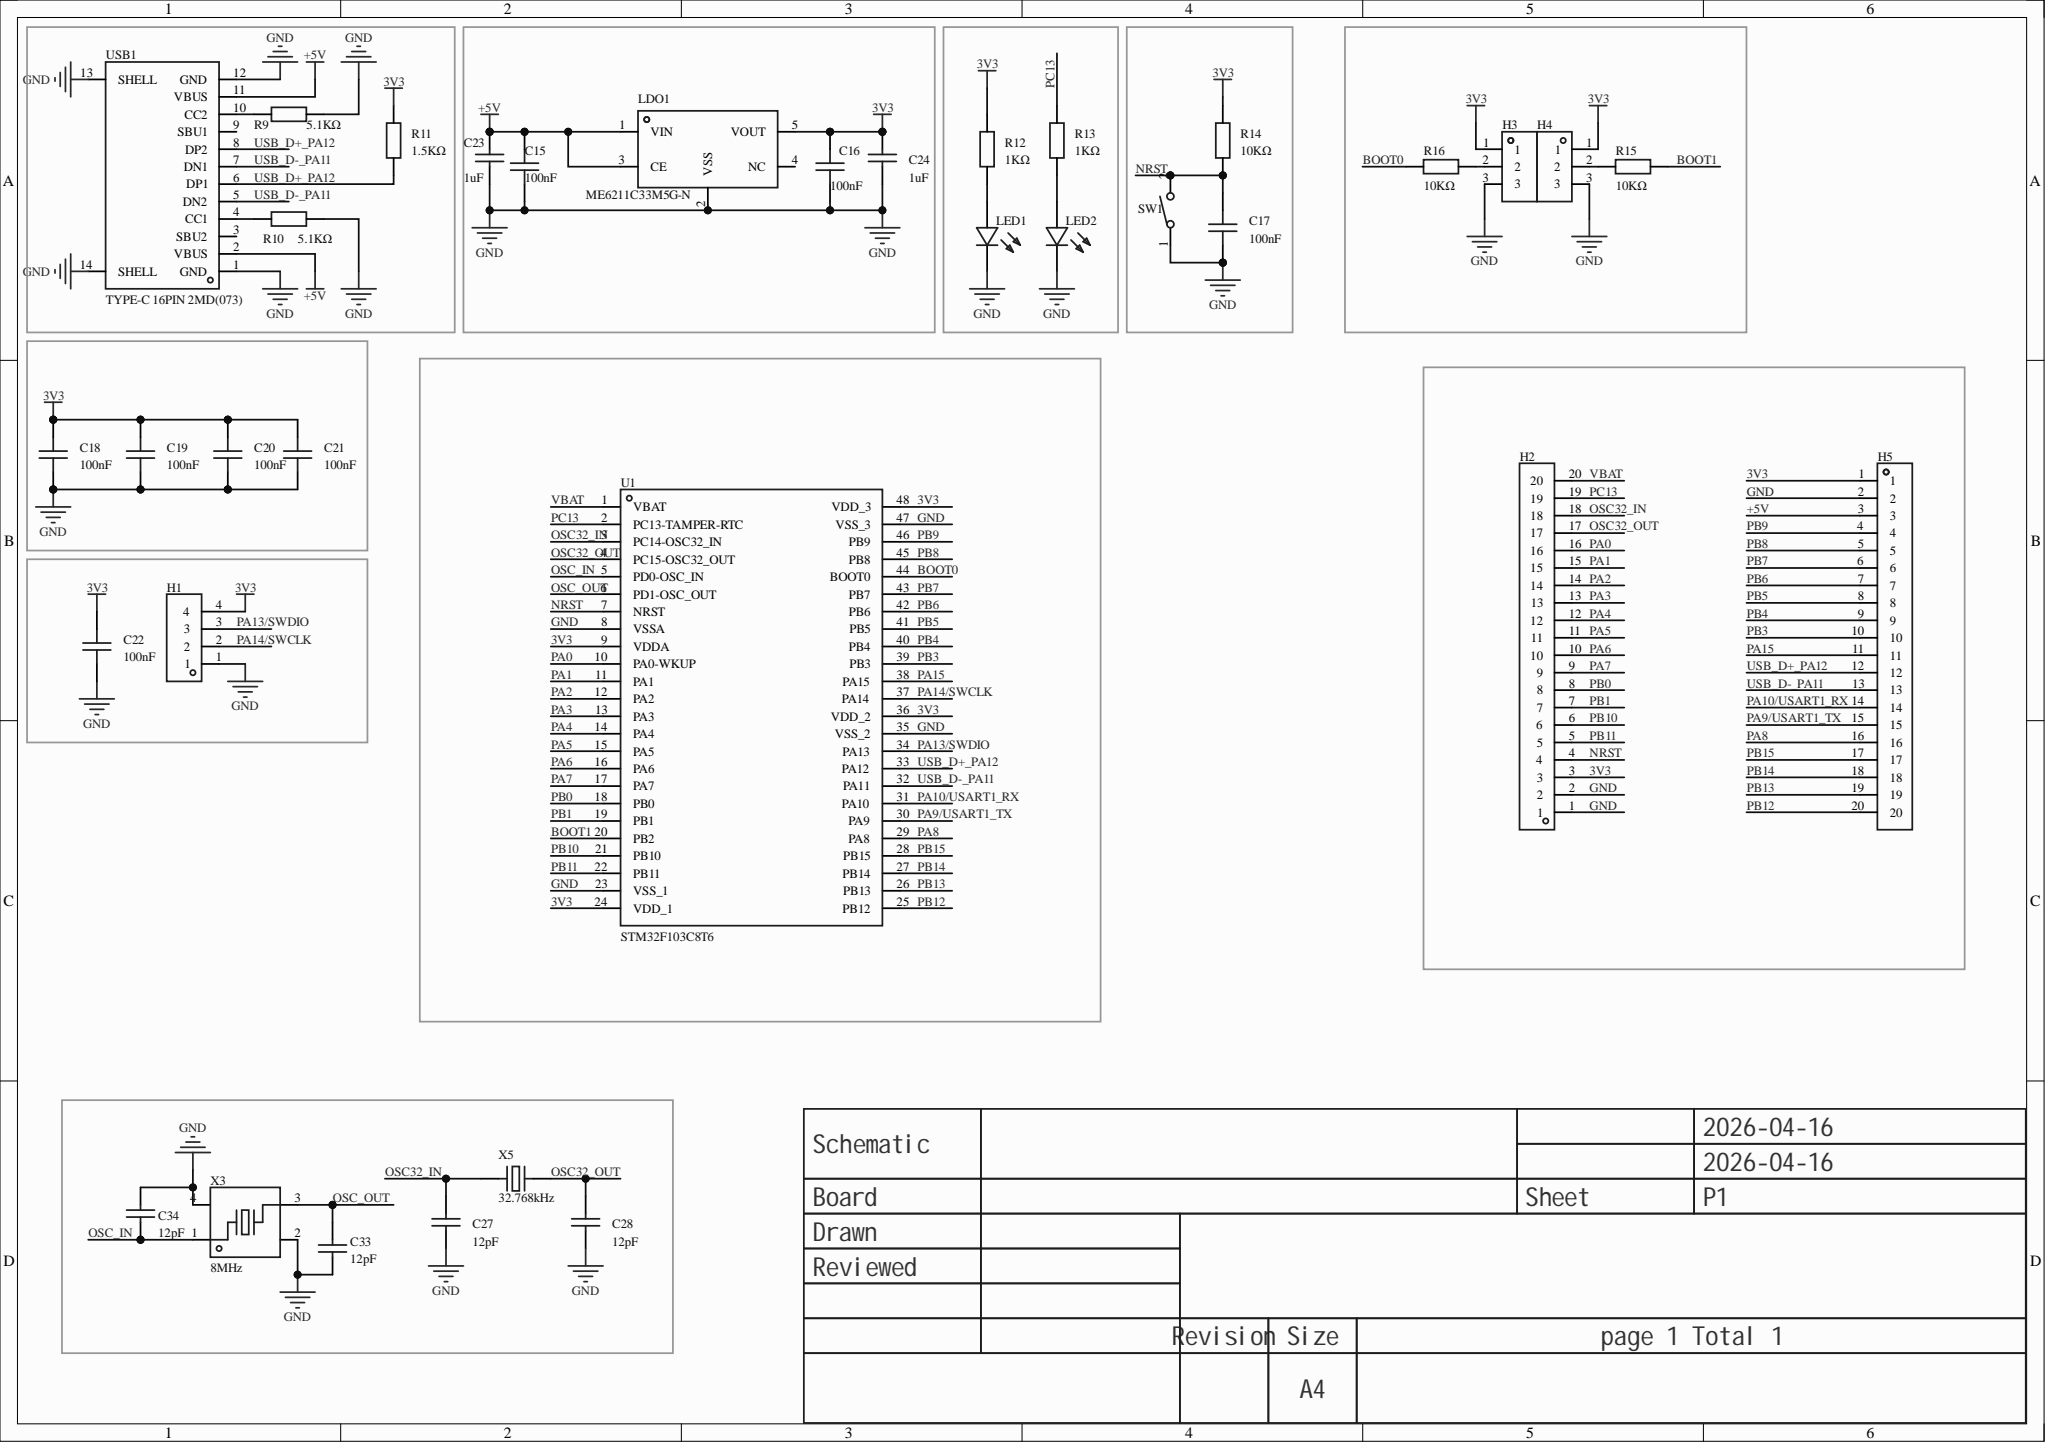Circuit board | Altium Designer | 35 parts | 49 nets
Bill of materials:
Comment,Description,Designator,Footprint,LibRef,Quantity
"100nF","Capacitance: 100nF; Tolerance: ±10%; Rated voltage: 50V; Temperature coefficient: X7R;","C15, C16, C17, C18, C19, C20, C21, C22","C0402","GRM155R71H104KE14D","8"
"1uF","Capacitance: 1uF; Tolerance: ±10%; Rated voltage: 10V; Temperature coefficient: X5R;","C23, C24","C0402","CL05A105KP5NNNC","2"
"12pF","Capacitance: 12pF; Tolerance: ±5%; Rated voltage: 50V; Temperature coefficient: C0G;","C27, C28, C33, C34","C0402","0402CG120J500NT","4"
"DZ254W-11-04-65","Pin structure: 1x4P; Pitch: 2.54mm; Row spacing: -; Round/square pins: Square pins; Mounting: Right-angle THT; Rows: Single row; Total pin count: 4P; Rated current: 3A; Rated voltage: -; Mating pin length: 6mm; Housing height: 2.54mm; Termination pin length: -; Contact material: Brass; Contact plating: Gold; Operating temperature: -; Color: Black;","H1","HDR-TH_4P-P2.54-H-M-W10.3","DZ254W-11-04-65","1"
"","Pitch: 2.54mm; Total pin count: 20; Rows: 1; Pin structure: -; Row spacing: -; Mounting type: Straight through-hole; Round/square pins: -; Rated current: -; Rated voltage: -; Mating pin length: -; Housing height: -; Contact material: Brass; Contact plating: -; Color: Black;","H2, H5","HDR-TH_20P-P2.54-V-M-1","HDR-M_2.54_1x20P","2"
"","","H3, H4","HDR-TH_3P-P2.54-V-M","HDR-M_2.54_1x3P","2"
"ME6211C33M5G-N","Output type: Fixed; Operating voltage: 6V; Output voltage: 3.3V; Output current: 500mA; Power supply rejection ratio (PSRR): 70dB@(1kHz); Output polarity: Positive;","LDO1","SOT-23-5_L3.0-W1.7-P0.95-LS2.8-BL","ME6211C33M5G-N","1"
"NCD0603R1","LED head type: -; Emission color: Red; Forward voltage (Vf): 1.6V~2.6V; Power: 65mW; Forward current: 25mA; Wavelength: 615nm~630nm; Diode configuration: Single diode; Lens color: -; Color temperature: -; Luminous intensity: 220mcd; Viewing angle: 130°; Tape packaging: -; Operating temperature: -30℃~+85℃;","LED1","LED0603-RD_RED","NCD0603R1_C84263","1"
"NCD0603B1","LED head type: -; Emission color: Blue; Forward voltage (Vf): 2.6V~3.6V; Power: 72mW; Forward current: 10mA; Wavelength: 463nm~475nm; Diode configuration: Single diode; Lens color: -; Color temperature: -; Luminous intensity: 220mcd; Viewing angle: 130°; Tape packaging: -; Operating temperature: -30℃~+85℃;","LED2","LED0603-RD","NCD0603B1","1"
"5.1KΩ","","R9, R10","R0805","Res_0805","2"
"1.5KΩ","","R11","R0805","Res_0805","1"
"1KΩ","","R12, R13","R0805","Res_0805","2"
"10KΩ","","R14, R15, R16","R0805","Res_0805","3"
"TS-1101-B-W","Circuit structure: SPST; Button shape: Rectangular button; Actuation force: 1.6N; Mounting: Upright mount; Switch length: 6mm; Switch width: 3.6mm; Switch height: 2.5mm; Bracket: Without bracket; Contact current: 50mA; Rated voltage: 12V; Lamp: None; Operating life: 5 wan cycles;","SW1","KEY-SMD_2P-L6.0-W3.6-P7.4-LS8.0-L","TS-1101-B-W_C500065","1"
"STM32F103C8T6","","U1","LQFP-48_L7.0-W7.0-P0.50-LS9.0-BL","STM32F103C8T6_C9900100366","1"
"TYPE-C 16PIN 2MD(073)","Connector type: Type-C; Protocol standard: -; Gender: Female; Mounting: Flat mount; Contacts: 16P; Ports: 1; Rated current - power: 3A; Operating temperature: -25℃~+85℃;","USB1","USB-C-SMD_TYPE-C-6PIN-2MD-073","TYPE-C 16PIN 2MD(073)","1"
"8MHz","Crystal type: SMD crystal; Frequency: 8MHz; Tolerance at room temp.: ±10ppm; Load capacitance: 12pF; Frequency stability: ±20ppm;","X3","CRYSTAL-SMD_4P-L3.2-W2.5-BL-1","XL2EL89COI-111YLC-8M","1"
"32.768kHz","Crystal type: SMD crystal; Frequency: 32.768kHz; Tolerance at room temp.: ±20ppm; Load capacitance: 12.5pF; Frequency stability: ±30ppm;","X5","OSC-SMD_L3.2-W1.5","X321532768KGD2SI","1"
Netlist (Protel format):
[
C15
C0402
100nF



]
[
C16
C0402
100nF



]
[
C17
C0402
100nF



]
[
C18
C0402
100nF



]
[
C19
C0402
100nF



]
[
C20
C0402
100nF



]
[
C21
C0402
100nF



]
[
C22
C0402
100nF



]
[
C23
C0402
1uF



]
[
C24
C0402
1uF



]
[
C27
C0402
12pF



]
[
C28
C0402
12pF



]
[
C33
C0402
12pF



]
[
C34
C0402
12pF



]
[
H1
HDR-TH_4P-P2.54-H-M-W10.3
DZ254W-11-04-65



]
[
H2
HDR-TH_20P-P2.54-V-M-1




]
[
H3
HDR-TH_3P-P2.54-V-M




]
[
H4
HDR-TH_3P-P2.54-V-M




]
[
H5
HDR-TH_20P-P2.54-V-M-1




]
[
LDO1
SOT-23-5_L3.0-W1.7-P0.95-LS2.8-BL
ME6211C33M5G-N



]
[
LED1
LED0603-RD_RED
NCD0603R1



]
[
LED2
LED0603-RD
NCD0603B1



]
[
R9
R0805
5.1KΩ



]
[
R10
R0805
5.1KΩ



]
[
R11
R0805
1.5KΩ



]
[
R12
R0805
1KΩ



]
[
R13
R0805
1KΩ



]
[
R14
R0805
10KΩ



]
[
R15
R0805
10KΩ



]
[
R16
R0805
10KΩ



]
[
SW1
KEY-SMD_2P-L6.0-W3.6-P7.4-LS8.0-L
TS-1101-B-W



]
[
U1
LQFP-48_L7.0-W7.0-P0.50-LS9.0-BL
STM32F103C8T6



]
[
USB1
USB-C-SMD_TYPE-C-6PIN-2MD-073
TYPE-C 16PIN 2MD(073)



]
[
X3
CRYSTAL-SMD_4P-L3.2-W2.5-BL-1
8MHz



]
[
X5
OSC-SMD_L3.2-W1.5
32.768kHz



]
(
VBAT
H2-20
U1-1
)
(
USB_D-_PA11
H5-13
U1-32
USB1-5
USB1-7
)
(
USB_D+_PA12
H5-12
R11-2
U1-33
USB1-6
USB1-8
)
(
PC13
H2-19
R13-2
U1-2
)
(
PB15
H5-17
U1-28
)
(
PB14
H5-18
U1-27
)
(
PB13
H5-19
U1-26
)
(
PB12
H5-20
U1-25
)
(
PB11
H2-5
U1-22
)
(
PB10
H2-6
U1-21
)
(
PB9
H5-4
U1-46
)
(
PB8
H5-5
U1-45
)
(
PB7
H5-6
U1-43
)
(
PB6
H5-7
U1-42
)
(
PB5
H5-8
U1-41
)
(
PB4
H5-9
U1-40
)
(
PB3
H5-10
U1-39
)
(
PB1
H2-7
U1-19
)
(
PB0
H2-8
U1-18
)
(
PA15
H5-11
U1-38
)
(
PA14/SWCLK
H1-2
U1-37
)
(
PA13/SWDIO
H1-3
U1-34
)
(
PA10/USART1_RX
H5-14
U1-31
)
(
PA9/USART1_TX
H5-15
U1-30
)
(
PA8
H5-16
U1-29
)
(
PA7
H2-9
U1-17
)
(
PA6
H2-10
U1-16
)
(
PA5
H2-11
U1-15
)
(
PA4
H2-12
U1-14
)
(
PA3
H2-13
U1-13
)
(
PA2
H2-14
U1-12
)
(
PA1
H2-15
U1-11
)
(
PA0
H2-16
U1-10
)
(
OSC_OUT
C33-2
U1-6
X3-3
)
(
OSC_IN
C34-1
U1-5
X3-1
)
(
OSC32_OUT
C28-2
H2-17
U1-4
X5-2
)
(
OSC32_IN
C27-2
H2-18
U1-3
X5-1
)
(
NRST
C17-2
H2-4
R14-1
SW1-2
U1-7
)
(
NetR10_1
R10-1
USB1-4
)
(
NetR9_1
R9-1
USB1-10
)
(
NetLED2_2
LED2-2
R13-1
)
(
NetLED1_2
LED1-2
R12-1
)
(
NetH4_2
H4-2
R15-1
)
(
NetH3_2
H3-2
R16-2
)
(
GND
C15-1
C16-1
C17-1
C18-1
C19-1
C20-1
C21-1
C22-1
C23-1
C24-1
C27-1
C28-1
C33-1
C34-2
H1-1
H2-1
H2-2
H3-3
H4-3
H5-2
LDO1-2
LED1-1
LED2-1
R9-2
R10-2
SW1-1
U1-8
U1-23
U1-35
U1-47
USB1-1
USB1-12
USB1-13
USB1-14
X3-2
X3-4
)
(
BOOT1
R15-2
U1-20
)
(
BOOT0
R16-1
U1-44
)
(
+5V
C15-2
C23-2
H5-3
LDO1-1
LDO1-3
USB1-2
USB1-11
)
(
3V3
C16-2
C18-2
C19-2
C20-2
C21-2
C22-2
C24-2
H1-4
H2-3
H3-1
H4-1
H5-1
LDO1-5
R11-1
R12-2
R14-2
U1-9
U1-24
U1-36
U1-48
)